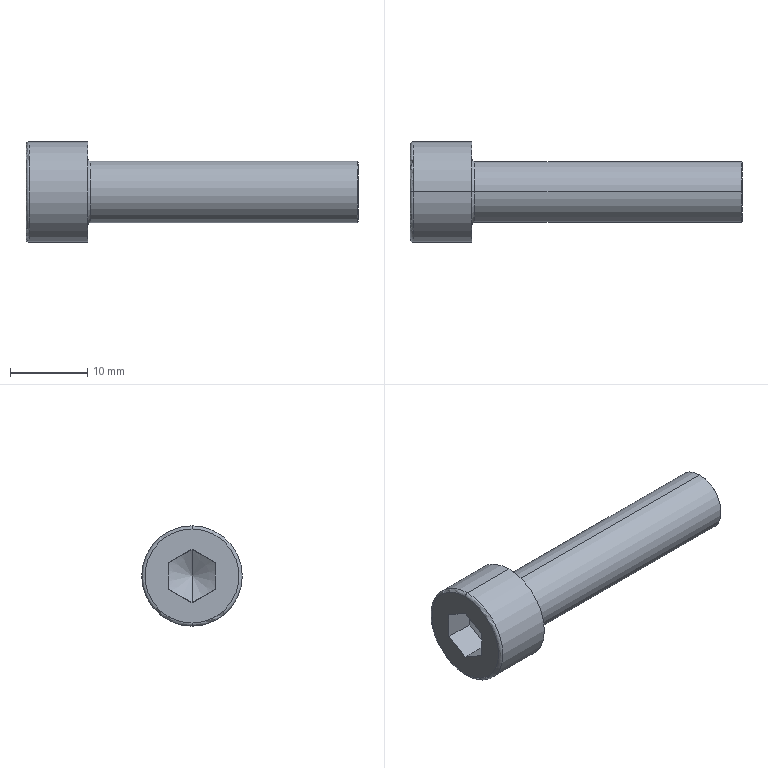Part | STEP file | 1 solid | 27 faces | box 43 x 13 x 13 mm | volume 2644 mm3 | plane 15 | torus 4 | cone 4 | cylinder 4 | commonest cylinder face diameters 7.92 x2 13 x2